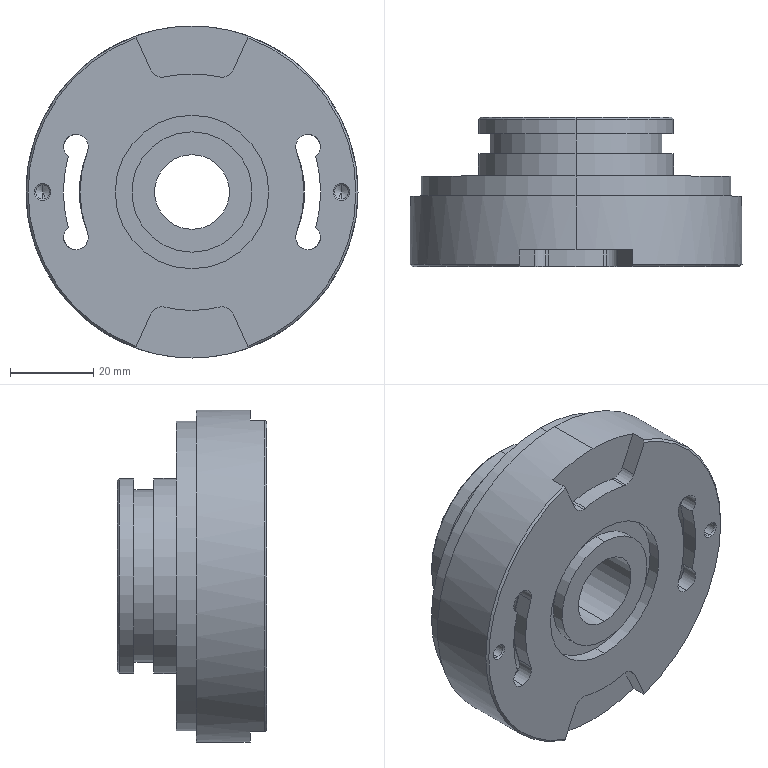Part | SolidWorks | features ICE 10, Chamfer 2, Extrusion 1, HoleWzd 1, MirrorPattern 1 | 1 solid | 96 faces | box 80 x 36 x 80 mm | volume 99071 mm3 | cylinder 43 | plane 29 | cone 24 | commonest cylinder face diameters 6 x12 3.3 x4 47 x4 57 x3 18 x2 29 x2